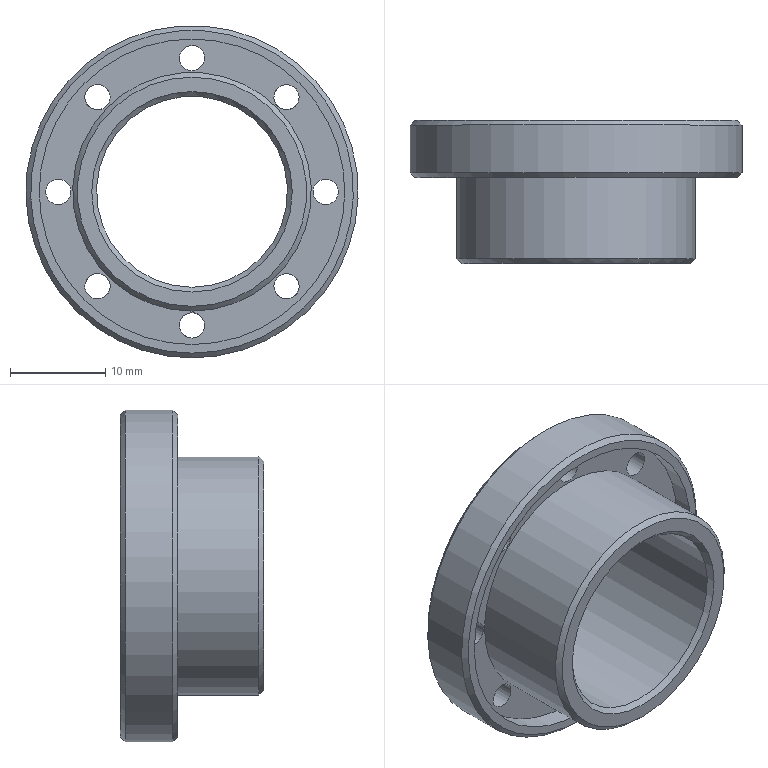Part | NX | features DATUM_CSYS 3, SKETCH 2, EXTRUDE 1, SWP104 1 | 1 solid | 21 faces | box 34.8 x 15 x 34.8 mm | volume 4556 mm3 | cylinder 12 | cone 5 | plane 4 | commonest cylinder face diameters 2.65 x8 20 x1 25 x1 32 x1 34.8 x1
STEP:
#1=CARTESIAN_POINT('',(0.,0.,-10.5));
#2=VERTEX_POINT('',#1);
#3=CARTESIAN_POINT('',(0.,0.,0.));
#4=DIRECTION('',(0.,-1.,0.));
#5=DIRECTION('',(0.,0.,-1.));
#6=AXIS2_PLACEMENT_3D('',#3,#4,#5);
#7=CIRCLE('',#6,10.5);
#8=EDGE_CURVE('',#2,#2,#7,.T.);
#9=ORIENTED_EDGE('',*,*,#8,.F.);
#10=EDGE_LOOP('',(#9));
#11=FACE_BOUND('',#10,.T.);
#12=CARTESIAN_POINT('',(0.,0.,-12.));
#13=VERTEX_POINT('',#12);
#14=CARTESIAN_POINT('',(0.,0.,0.));
#15=DIRECTION('',(0.,-1.,0.));
#16=DIRECTION('',(0.,0.,-1.));
#17=AXIS2_PLACEMENT_3D('',#14,#15,#16);
#18=CIRCLE('',#17,12.);
#19=EDGE_CURVE('',#13,#13,#18,.T.);
#20=ORIENTED_EDGE('',*,*,#19,.T.);
#21=EDGE_LOOP('',(#20));
#22=FACE_BOUND('',#21,.T.);
#23=CARTESIAN_POINT('',(0.,0.,12.));
#24=DIRECTION('',(0.,1.,0.));
#25=DIRECTION('',(0.,0.,1.));
#26=AXIS2_PLACEMENT_3D('',#23,#24,#25);
#27=PLANE('',#26);
#28=ADVANCED_FACE('',(#11,#22),#27,.F.);
#29=CARTESIAN_POINT('',(0.,0.5,-10.));
#30=VERTEX_POINT('',#29);
#31=CARTESIAN_POINT('',(0.,0.5,0.));
#32=DIRECTION('',(0.,-1.,0.));
#33=DIRECTION('',(0.,0.,-1.));
#34=AXIS2_PLACEMENT_3D('',#31,#32,#33);
#35=CIRCLE('',#34,10.);
#36=EDGE_CURVE('',#30,#30,#35,.T.);
#37=ORIENTED_EDGE('',*,*,#36,.F.);
#38=EDGE_LOOP('',(#37));
#39=FACE_BOUND('',#38,.T.);
#40=ORIENTED_EDGE('',*,*,#8,.T.);
#41=EDGE_LOOP('',(#40));
#42=FACE_BOUND('',#41,.T.);
#43=CARTESIAN_POINT('',(0.,0.,0.));
#44=DIRECTION('',(0.,-1.,0.));
#45=DIRECTION('',(0.,0.,-1.));
#46=AXIS2_PLACEMENT_3D('',#43,#44,#45);
#47=CONICAL_SURFACE('',#46,10.5,0.7854);
#48=ADVANCED_FACE('',(#39,#42),#47,.F.);
#49=CARTESIAN_POINT('',(0.,14.5,-10.));
#50=VERTEX_POINT('',#49);
#51=CARTESIAN_POINT('',(0.,14.5,0.));
#52=DIRECTION('',(0.,-1.,0.));
#53=DIRECTION('',(0.,0.,-1.));
#54=AXIS2_PLACEMENT_3D('',#51,#52,#53);
#55=CIRCLE('',#54,10.);
#56=EDGE_CURVE('',#50,#50,#55,.T.);
#57=ORIENTED_EDGE('',*,*,#56,.F.);
#58=EDGE_LOOP('',(#57));
#59=FACE_BOUND('',#58,.T.);
#60=ORIENTED_EDGE('',*,*,#36,.T.);
#61=EDGE_LOOP('',(#60));
#62=FACE_BOUND('',#61,.T.);
#63=CARTESIAN_POINT('',(0.,0.,0.));
#64=DIRECTION('',(0.,-1.,0.));
#65=DIRECTION('',(0.,0.,-1.));
#66=AXIS2_PLACEMENT_3D('',#63,#64,#65);
#67=CYLINDRICAL_SURFACE('',#66,10.);
#68=ADVANCED_FACE('',(#59,#62),#67,.F.);
#69=CARTESIAN_POINT('',(0.,15.,-10.5));
#70=VERTEX_POINT('',#69);
#71=CARTESIAN_POINT('',(0.,15.,0.));
#72=DIRECTION('',(0.,-1.,0.));
#73=DIRECTION('',(0.,0.,-1.));
#74=AXIS2_PLACEMENT_3D('',#71,#72,#73);
#75=CIRCLE('',#74,10.5);
#76=EDGE_CURVE('',#70,#70,#75,.T.);
#77=ORIENTED_EDGE('',*,*,#76,.F.);
#78=EDGE_LOOP('',(#77));
#79=FACE_BOUND('',#78,.T.);
#80=ORIENTED_EDGE('',*,*,#56,.T.);
#81=EDGE_LOOP('',(#80));
#82=FACE_BOUND('',#81,.T.);
#83=CARTESIAN_POINT('',(0.,14.5,0.));
#84=DIRECTION('',(0.,1.,0.));
#85=DIRECTION('',(0.,0.,1.));
#86=AXIS2_PLACEMENT_3D('',#83,#84,#85);
#87=CONICAL_SURFACE('',#86,10.,0.7854);
#88=ADVANCED_FACE('',(#79,#82),#87,.F.);
#89=CARTESIAN_POINT('',(14.,15.,-1.325));
#90=VERTEX_POINT('',#89);
#91=CARTESIAN_POINT('',(14.,15.,0.));
#92=DIRECTION('',(0.,-1.,0.));
#93=DIRECTION('',(0.,0.,-1.));
#94=AXIS2_PLACEMENT_3D('',#91,#92,#93);
#95=CIRCLE('',#94,1.325);
#96=EDGE_CURVE('',#90,#90,#95,.T.);
#97=ORIENTED_EDGE('',*,*,#96,.T.);
#98=EDGE_LOOP('',(#97));
#99=FACE_BOUND('',#98,.T.);
#100=CARTESIAN_POINT('',(9.899,15.,-11.224));
#101=VERTEX_POINT('',#100);
#102=CARTESIAN_POINT('',(9.899,15.,-9.899));
#103=DIRECTION('',(0.,-1.,0.));
#104=DIRECTION('',(0.,0.,-1.));
#105=AXIS2_PLACEMENT_3D('',#102,#103,#104);
#106=CIRCLE('',#105,1.325);
#107=EDGE_CURVE('',#101,#101,#106,.T.);
#108=ORIENTED_EDGE('',*,*,#107,.T.);
#109=EDGE_LOOP('',(#108));
#110=FACE_BOUND('',#109,.T.);
#111=CARTESIAN_POINT('',(0.,15.,-15.325));
#112=VERTEX_POINT('',#111);
#113=CARTESIAN_POINT('',(0.,15.,-14.));
#114=DIRECTION('',(0.,-1.,0.));
#115=DIRECTION('',(0.,0.,-1.));
#116=AXIS2_PLACEMENT_3D('',#113,#114,#115);
#117=CIRCLE('',#116,1.325);
#118=EDGE_CURVE('',#112,#112,#117,.T.);
#119=ORIENTED_EDGE('',*,*,#118,.T.);
#120=EDGE_LOOP('',(#119));
#121=FACE_BOUND('',#120,.T.);
#122=CARTESIAN_POINT('',(-9.899,15.,-11.224));
#123=VERTEX_POINT('',#122);
#124=CARTESIAN_POINT('',(-9.899,15.,-9.899));
#125=DIRECTION('',(0.,-1.,0.));
#126=DIRECTION('',(0.,0.,-1.));
#127=AXIS2_PLACEMENT_3D('',#124,#125,#126);
#128=CIRCLE('',#127,1.325);
#129=EDGE_CURVE('',#123,#123,#128,.T.);
#130=ORIENTED_EDGE('',*,*,#129,.T.);
#131=EDGE_LOOP('',(#130));
#132=FACE_BOUND('',#131,.T.);
#133=CARTESIAN_POINT('',(-14.,15.,-1.325));
#134=VERTEX_POINT('',#133);
#135=CARTESIAN_POINT('',(-14.,15.,0.));
#136=DIRECTION('',(0.,-1.,0.));
#137=DIRECTION('',(0.,0.,-1.));
#138=AXIS2_PLACEMENT_3D('',#135,#136,#137);
#139=CIRCLE('',#138,1.325);
#140=EDGE_CURVE('',#134,#134,#139,.T.);
#141=ORIENTED_EDGE('',*,*,#140,.T.);
#142=EDGE_LOOP('',(#141));
#143=FACE_BOUND('',#142,.T.);
#144=CARTESIAN_POINT('',(-9.899,15.,8.574));
#145=VERTEX_POINT('',#144);
#146=CARTESIAN_POINT('',(-9.899,15.,9.899));
#147=DIRECTION('',(0.,-1.,0.));
#148=DIRECTION('',(0.,0.,-1.));
#149=AXIS2_PLACEMENT_3D('',#146,#147,#148);
#150=CIRCLE('',#149,1.325);
#151=EDGE_CURVE('',#145,#145,#150,.T.);
#152=ORIENTED_EDGE('',*,*,#151,.T.);
#153=EDGE_LOOP('',(#152));
#154=FACE_BOUND('',#153,.T.);
#155=CARTESIAN_POINT('',(0.,15.,12.675));
#156=VERTEX_POINT('',#155);
#157=CARTESIAN_POINT('',(0.,15.,14.));
#158=DIRECTION('',(0.,-1.,0.));
#159=DIRECTION('',(0.,0.,-1.));
#160=AXIS2_PLACEMENT_3D('',#157,#158,#159);
#161=CIRCLE('',#160,1.325);
#162=EDGE_CURVE('',#156,#156,#161,.T.);
#163=ORIENTED_EDGE('',*,*,#162,.T.);
#164=EDGE_LOOP('',(#163));
#165=FACE_BOUND('',#164,.T.);
#166=CARTESIAN_POINT('',(9.899,15.,8.574));
#167=VERTEX_POINT('',#166);
#168=CARTESIAN_POINT('',(9.899,15.,9.899));
#169=DIRECTION('',(0.,-1.,0.));
#170=DIRECTION('',(0.,0.,-1.));
#171=AXIS2_PLACEMENT_3D('',#168,#169,#170);
#172=CIRCLE('',#171,1.325);
#173=EDGE_CURVE('',#167,#167,#172,.T.);
#174=ORIENTED_EDGE('',*,*,#173,.T.);
#175=EDGE_LOOP('',(#174));
#176=FACE_BOUND('',#175,.T.);
#177=CARTESIAN_POINT('',(0.,15.,-16.9));
#178=VERTEX_POINT('',#177);
#179=CARTESIAN_POINT('',(0.,15.,0.));
#180=DIRECTION('',(0.,-1.,0.));
#181=DIRECTION('',(0.,0.,-1.));
#182=AXIS2_PLACEMENT_3D('',#179,#180,#181);
#183=CIRCLE('',#182,16.9);
#184=EDGE_CURVE('',#178,#178,#183,.T.);
#185=ORIENTED_EDGE('',*,*,#184,.F.);
#186=EDGE_LOOP('',(#185));
#187=FACE_BOUND('',#186,.T.);
#188=ORIENTED_EDGE('',*,*,#76,.T.);
#189=EDGE_LOOP('',(#188));
#190=FACE_BOUND('',#189,.T.);
#191=CARTESIAN_POINT('',(0.,15.,10.5));
#192=DIRECTION('',(0.,-1.,0.));
#193=DIRECTION('',(0.,0.,-1.));
#194=AXIS2_PLACEMENT_3D('',#191,#192,#193);
#195=PLANE('',#194);
#196=ADVANCED_FACE('',(#99,#110,#121,#132,#143,#154,#165,#176,#187,#190),#195,.F.);
#197=CARTESIAN_POINT('',(0.,14.5,-17.4));
#198=VERTEX_POINT('',#197);
#199=CARTESIAN_POINT('',(0.,14.5,0.));
#200=DIRECTION('',(0.,-1.,0.));
#201=DIRECTION('',(0.,0.,-1.));
#202=AXIS2_PLACEMENT_3D('',#199,#200,#201);
#203=CIRCLE('',#202,17.4);
#204=EDGE_CURVE('',#198,#198,#203,.T.);
#205=ORIENTED_EDGE('',*,*,#204,.F.);
#206=EDGE_LOOP('',(#205));
#207=FACE_BOUND('',#206,.T.);
#208=ORIENTED_EDGE('',*,*,#184,.T.);
#209=EDGE_LOOP('',(#208));
#210=FACE_BOUND('',#209,.T.);
#211=CARTESIAN_POINT('',(0.,15.,0.));
#212=DIRECTION('',(0.,-1.,0.));
#213=DIRECTION('',(0.,0.,-1.));
#214=AXIS2_PLACEMENT_3D('',#211,#212,#213);
#215=CONICAL_SURFACE('',#214,16.9,0.7854);
#216=ADVANCED_FACE('',(#207,#210),#215,.T.);
#217=CARTESIAN_POINT('',(0.,9.5,-17.4));
#218=VERTEX_POINT('',#217);
#219=CARTESIAN_POINT('',(0.,9.5,0.));
#220=DIRECTION('',(0.,-1.,0.));
#221=DIRECTION('',(0.,0.,-1.));
#222=AXIS2_PLACEMENT_3D('',#219,#220,#221);
#223=CIRCLE('',#222,17.4);
#224=EDGE_CURVE('',#218,#218,#223,.T.);
#225=ORIENTED_EDGE('',*,*,#224,.F.);
#226=EDGE_LOOP('',(#225));
#227=FACE_BOUND('',#226,.T.);
#228=ORIENTED_EDGE('',*,*,#204,.T.);
#229=EDGE_LOOP('',(#228));
#230=FACE_BOUND('',#229,.T.);
#231=CARTESIAN_POINT('',(0.,0.,0.));
#232=DIRECTION('',(0.,-1.,0.));
#233=DIRECTION('',(0.,0.,-1.));
#234=AXIS2_PLACEMENT_3D('',#231,#232,#233);
#235=CYLINDRICAL_SURFACE('',#234,17.4);
#236=ADVANCED_FACE('',(#227,#230),#235,.T.);
#237=CARTESIAN_POINT('',(0.,9.,-16.9));
#238=VERTEX_POINT('',#237);
#239=CARTESIAN_POINT('',(0.,9.,0.));
#240=DIRECTION('',(0.,-1.,0.));
#241=DIRECTION('',(0.,0.,-1.));
#242=AXIS2_PLACEMENT_3D('',#239,#240,#241);
#243=CIRCLE('',#242,16.9);
#244=EDGE_CURVE('',#238,#238,#243,.T.);
#245=ORIENTED_EDGE('',*,*,#244,.F.);
#246=EDGE_LOOP('',(#245));
#247=FACE_BOUND('',#246,.T.);
#248=ORIENTED_EDGE('',*,*,#224,.T.);
#249=EDGE_LOOP('',(#248));
#250=FACE_BOUND('',#249,.T.);
#251=CARTESIAN_POINT('',(0.,9.5,0.));
#252=DIRECTION('',(0.,1.,0.));
#253=DIRECTION('',(0.,0.,1.));
#254=AXIS2_PLACEMENT_3D('',#251,#252,#253);
#255=CONICAL_SURFACE('',#254,17.4,0.7854);
#256=ADVANCED_FACE('',(#247,#250),#255,.T.);
#257=CARTESIAN_POINT('',(0.,9.,-16.));
#258=VERTEX_POINT('',#257);
#259=CARTESIAN_POINT('',(0.,9.,0.));
#260=DIRECTION('',(0.,-1.,0.));
#261=DIRECTION('',(0.,0.,-1.));
#262=AXIS2_PLACEMENT_3D('',#259,#260,#261);
#263=CIRCLE('',#262,16.);
#264=EDGE_CURVE('',#258,#258,#263,.T.);
#265=ORIENTED_EDGE('',*,*,#264,.F.);
#266=EDGE_LOOP('',(#265));
#267=FACE_BOUND('',#266,.T.);
#268=ORIENTED_EDGE('',*,*,#244,.T.);
#269=EDGE_LOOP('',(#268));
#270=FACE_BOUND('',#269,.T.);
#271=CARTESIAN_POINT('',(0.,9.,16.9));
#272=DIRECTION('',(0.,1.,0.));
#273=DIRECTION('',(0.,0.,1.));
#274=AXIS2_PLACEMENT_3D('',#271,#272,#273);
#275=PLANE('',#274);
#276=ADVANCED_FACE('',(#267,#270),#275,.F.);
#277=CARTESIAN_POINT('',(0.,11.,-16.));
#278=VERTEX_POINT('',#277);
#279=CARTESIAN_POINT('',(0.,11.,0.));
#280=DIRECTION('',(0.,-1.,0.));
#281=DIRECTION('',(0.,0.,-1.));
#282=AXIS2_PLACEMENT_3D('',#279,#280,#281);
#283=CIRCLE('',#282,16.);
#284=EDGE_CURVE('',#278,#278,#283,.T.);
#285=ORIENTED_EDGE('',*,*,#284,.F.);
#286=EDGE_LOOP('',(#285));
#287=FACE_BOUND('',#286,.T.);
#288=ORIENTED_EDGE('',*,*,#264,.T.);
#289=EDGE_LOOP('',(#288));
#290=FACE_BOUND('',#289,.T.);
#291=CARTESIAN_POINT('',(0.,0.,0.));
#292=DIRECTION('',(0.,-1.,0.));
#293=DIRECTION('',(0.,0.,-1.));
#294=AXIS2_PLACEMENT_3D('',#291,#292,#293);
#295=CYLINDRICAL_SURFACE('',#294,16.);
#296=ADVANCED_FACE('',(#287,#290),#295,.F.);
#297=CARTESIAN_POINT('',(14.,11.,-1.325));
#298=VERTEX_POINT('',#297);
#299=CARTESIAN_POINT('',(14.,11.,0.));
#300=DIRECTION('',(0.,-1.,0.));
#301=DIRECTION('',(0.,0.,-1.));
#302=AXIS2_PLACEMENT_3D('',#299,#300,#301);
#303=CIRCLE('',#302,1.325);
#304=EDGE_CURVE('',#298,#298,#303,.T.);
#305=ORIENTED_EDGE('',*,*,#304,.F.);
#306=EDGE_LOOP('',(#305));
#307=FACE_BOUND('',#306,.T.);
#308=CARTESIAN_POINT('',(8.963,11.,-10.836));
#309=VERTEX_POINT('',#308);
#310=CARTESIAN_POINT('',(9.899,11.,-9.899));
#311=DIRECTION('',(0.,-1.,0.));
#312=DIRECTION('',(-0.7071,0.,-0.7071));
#313=AXIS2_PLACEMENT_3D('',#310,#311,#312);
#314=CIRCLE('',#313,1.325);
#315=EDGE_CURVE('',#309,#309,#314,.T.);
#316=ORIENTED_EDGE('',*,*,#315,.F.);
#317=EDGE_LOOP('',(#316));
#318=FACE_BOUND('',#317,.T.);
#319=CARTESIAN_POINT('',(-1.325,11.,-14.));
#320=VERTEX_POINT('',#319);
#321=CARTESIAN_POINT('',(0.,11.,-14.));
#322=DIRECTION('',(0.,-1.,0.));
#323=DIRECTION('',(-1.,0.,0.));
#324=AXIS2_PLACEMENT_3D('',#321,#322,#323);
#325=CIRCLE('',#324,1.325);
#326=EDGE_CURVE('',#320,#320,#325,.T.);
#327=ORIENTED_EDGE('',*,*,#326,.F.);
#328=EDGE_LOOP('',(#327));
#329=FACE_BOUND('',#328,.T.);
#330=CARTESIAN_POINT('',(-10.836,11.,-8.963));
#331=VERTEX_POINT('',#330);
#332=CARTESIAN_POINT('',(-9.899,11.,-9.899));
#333=DIRECTION('',(0.,-1.,0.));
#334=DIRECTION('',(-0.7071,0.,0.7071));
#335=AXIS2_PLACEMENT_3D('',#332,#333,#334);
#336=CIRCLE('',#335,1.325);
#337=EDGE_CURVE('',#331,#331,#336,.T.);
#338=ORIENTED_EDGE('',*,*,#337,.F.);
#339=EDGE_LOOP('',(#338));
#340=FACE_BOUND('',#339,.T.);
#341=CARTESIAN_POINT('',(-14.,11.,1.325));
#342=VERTEX_POINT('',#341);
#343=CARTESIAN_POINT('',(-14.,11.,0.));
#344=DIRECTION('',(0.,-1.,0.));
#345=DIRECTION('',(0.,0.,1.));
#346=AXIS2_PLACEMENT_3D('',#343,#344,#345);
#347=CIRCLE('',#346,1.325);
#348=EDGE_CURVE('',#342,#342,#347,.T.);
#349=ORIENTED_EDGE('',*,*,#348,.F.);
#350=EDGE_LOOP('',(#349));
#351=FACE_BOUND('',#350,.T.);
#352=CARTESIAN_POINT('',(-8.963,11.,10.836));
#353=VERTEX_POINT('',#352);
#354=CARTESIAN_POINT('',(-9.899,11.,9.899));
#355=DIRECTION('',(0.,-1.,0.));
#356=DIRECTION('',(0.7071,0.,0.7071));
#357=AXIS2_PLACEMENT_3D('',#354,#355,#356);
#358=CIRCLE('',#357,1.325);
#359=EDGE_CURVE('',#353,#353,#358,.T.);
#360=ORIENTED_EDGE('',*,*,#359,.F.);
#361=EDGE_LOOP('',(#360));
#362=FACE_BOUND('',#361,.T.);
#363=CARTESIAN_POINT('',(1.325,11.,14.));
#364=VERTEX_POINT('',#363);
#365=CARTESIAN_POINT('',(0.,11.,14.));
#366=DIRECTION('',(0.,-1.,0.));
#367=DIRECTION('',(1.,0.,0.));
#368=AXIS2_PLACEMENT_3D('',#365,#366,#367);
#369=CIRCLE('',#368,1.325);
#370=EDGE_CURVE('',#364,#364,#369,.T.);
#371=ORIENTED_EDGE('',*,*,#370,.F.);
#372=EDGE_LOOP('',(#371));
#373=FACE_BOUND('',#372,.T.);
#374=CARTESIAN_POINT('',(10.836,11.,8.963));
#375=VERTEX_POINT('',#374);
#376=CARTESIAN_POINT('',(9.899,11.,9.899));
#377=DIRECTION('',(0.,-1.,0.));
#378=DIRECTION('',(0.7071,0.,-0.7071));
#379=AXIS2_PLACEMENT_3D('',#376,#377,#378);
#380=CIRCLE('',#379,1.325);
#381=EDGE_CURVE('',#375,#375,#380,.T.);
#382=ORIENTED_EDGE('',*,*,#381,.F.);
#383=EDGE_LOOP('',(#382));
#384=FACE_BOUND('',#383,.T.);
#385=CARTESIAN_POINT('',(0.,11.,-12.5));
#386=VERTEX_POINT('',#385);
#387=CARTESIAN_POINT('',(0.,11.,0.));
#388=DIRECTION('',(0.,-1.,0.));
#389=DIRECTION('',(0.,0.,-1.));
#390=AXIS2_PLACEMENT_3D('',#387,#388,#389);
#391=CIRCLE('',#390,12.5);
#392=EDGE_CURVE('',#386,#386,#391,.T.);
#393=ORIENTED_EDGE('',*,*,#392,.F.);
#394=EDGE_LOOP('',(#393));
#395=FACE_BOUND('',#394,.T.);
#396=ORIENTED_EDGE('',*,*,#284,.T.);
#397=EDGE_LOOP('',(#396));
#398=FACE_BOUND('',#397,.T.);
#399=CARTESIAN_POINT('',(0.,11.,16.));
#400=DIRECTION('',(0.,1.,0.));
#401=DIRECTION('',(0.,0.,1.));
#402=AXIS2_PLACEMENT_3D('',#399,#400,#401);
#403=PLANE('',#402);
#404=ADVANCED_FACE('',(#307,#318,#329,#340,#351,#362,#373,#384,#395,#398),#403,.F.);
#405=CARTESIAN_POINT('',(0.,0.5,-12.5));
#406=VERTEX_POINT('',#405);
#407=CARTESIAN_POINT('',(0.,0.5,0.));
#408=DIRECTION('',(0.,-1.,0.));
#409=DIRECTION('',(0.,0.,-1.));
#410=AXIS2_PLACEMENT_3D('',#407,#408,#409);
#411=CIRCLE('',#410,12.5);
#412=EDGE_CURVE('',#406,#406,#411,.T.);
#413=ORIENTED_EDGE('',*,*,#412,.F.);
#414=EDGE_LOOP('',(#413));
#415=FACE_BOUND('',#414,.T.);
#416=ORIENTED_EDGE('',*,*,#392,.T.);
#417=EDGE_LOOP('',(#416));
#418=FACE_BOUND('',#417,.T.);
#419=CARTESIAN_POINT('',(0.,0.,0.));
#420=DIRECTION('',(0.,-1.,0.));
#421=DIRECTION('',(0.,0.,-1.));
#422=AXIS2_PLACEMENT_3D('',#419,#420,#421);
#423=CYLINDRICAL_SURFACE('',#422,12.5);
#424=ADVANCED_FACE('',(#415,#418),#423,.T.);
#425=ORIENTED_EDGE('',*,*,#19,.F.);
#426=EDGE_LOOP('',(#425));
#427=FACE_BOUND('',#426,.T.);
#428=ORIENTED_EDGE('',*,*,#412,.T.);
#429=EDGE_LOOP('',(#428));
#430=FACE_BOUND('',#429,.T.);
#431=CARTESIAN_POINT('',(0.,0.5,0.));
#432=DIRECTION('',(0.,1.,0.));
#433=DIRECTION('',(0.,0.,1.));
#434=AXIS2_PLACEMENT_3D('',#431,#432,#433);
#435=CONICAL_SURFACE('',#434,12.5,0.7854);
#436=ADVANCED_FACE('',(#427,#430),#435,.T.);
#437=ORIENTED_EDGE('',*,*,#381,.T.);
#438=EDGE_LOOP('',(#437));
#439=FACE_BOUND('',#438,.T.);
#440=ORIENTED_EDGE('',*,*,#173,.F.);
#441=EDGE_LOOP('',(#440));
#442=FACE_BOUND('',#441,.T.);
#443=CARTESIAN_POINT('',(9.899,30.,9.899));
#444=DIRECTION('',(0.,-1.,0.));
#445=DIRECTION('',(0.,0.,-1.));
#446=AXIS2_PLACEMENT_3D('',#443,#444,#445);
#447=CYLINDRICAL_SURFACE('',#446,1.325);
#448=ADVANCED_FACE('',(#439,#442),#447,.F.);
#449=ORIENTED_EDGE('',*,*,#370,.T.);
#450=EDGE_LOOP('',(#449));
#451=FACE_BOUND('',#450,.T.);
#452=ORIENTED_EDGE('',*,*,#162,.F.);
#453=EDGE_LOOP('',(#452));
#454=FACE_BOUND('',#453,.T.);
#455=CARTESIAN_POINT('',(0.,30.,14.));
#456=DIRECTION('',(0.,-1.,0.));
#457=DIRECTION('',(0.,0.,-1.));
#458=AXIS2_PLACEMENT_3D('',#455,#456,#457);
#459=CYLINDRICAL_SURFACE('',#458,1.325);
#460=ADVANCED_FACE('',(#451,#454),#459,.F.);
#461=ORIENTED_EDGE('',*,*,#359,.T.);
#462=EDGE_LOOP('',(#461));
#463=FACE_BOUND('',#462,.T.);
#464=ORIENTED_EDGE('',*,*,#151,.F.);
#465=EDGE_LOOP('',(#464));
#466=FACE_BOUND('',#465,.T.);
#467=CARTESIAN_POINT('',(-9.899,30.,9.899));
#468=DIRECTION('',(0.,-1.,0.));
#469=DIRECTION('',(0.,0.,-1.));
#470=AXIS2_PLACEMENT_3D('',#467,#468,#469);
#471=CYLINDRICAL_SURFACE('',#470,1.325);
#472=ADVANCED_FACE('',(#463,#466),#471,.F.);
#473=ORIENTED_EDGE('',*,*,#348,.T.);
#474=EDGE_LOOP('',(#473));
#475=FACE_BOUND('',#474,.T.);
#476=ORIENTED_EDGE('',*,*,#140,.F.);
#477=EDGE_LOOP('',(#476));
#478=FACE_BOUND('',#477,.T.);
#479=CARTESIAN_POINT('',(-14.,30.,0.));
#480=DIRECTION('',(0.,-1.,0.));
#481=DIRECTION('',(0.,0.,-1.));
#482=AXIS2_PLACEMENT_3D('',#479,#480,#481);
#483=CYLINDRICAL_SURFACE('',#482,1.325);
#484=ADVANCED_FACE('',(#475,#478),#483,.F.);
#485=ORIENTED_EDGE('',*,*,#337,.T.);
#486=EDGE_LOOP('',(#485));
#487=FACE_BOUND('',#486,.T.);
#488=ORIENTED_EDGE('',*,*,#129,.F.);
#489=EDGE_LOOP('',(#488));
#490=FACE_BOUND('',#489,.T.);
#491=CARTESIAN_POINT('',(-9.899,30.,-9.899));
#492=DIRECTION('',(0.,-1.,0.));
#493=DIRECTION('',(0.,0.,-1.));
#494=AXIS2_PLACEMENT_3D('',#491,#492,#493);
#495=CYLINDRICAL_SURFACE('',#494,1.325);
#496=ADVANCED_FACE('',(#487,#490),#495,.F.);
#497=ORIENTED_EDGE('',*,*,#326,.T.);
#498=EDGE_LOOP('',(#497));
#499=FACE_BOUND('',#498,.T.);
#500=ORIENTED_EDGE('',*,*,#118,.F.);
#501=EDGE_LOOP('',(#500));
#502=FACE_BOUND('',#501,.T.);
#503=CARTESIAN_POINT('',(0.,30.,-14.));
#504=DIRECTION('',(0.,-1.,0.));
#505=DIRECTION('',(0.,0.,-1.));
#506=AXIS2_PLACEMENT_3D('',#503,#504,#505);
#507=CYLINDRICAL_SURFACE('',#506,1.325);
#508=ADVANCED_FACE('',(#499,#502),#507,.F.);
#509=ORIENTED_EDGE('',*,*,#315,.T.);
#510=EDGE_LOOP('',(#509));
#511=FACE_BOUND('',#510,.T.);
#512=ORIENTED_EDGE('',*,*,#107,.F.);
#513=EDGE_LOOP('',(#512));
#514=FACE_BOUND('',#513,.T.);
#515=CARTESIAN_POINT('',(9.899,30.,-9.899));
#516=DIRECTION('',(0.,-1.,0.));
#517=DIRECTION('',(0.,0.,-1.));
#518=AXIS2_PLACEMENT_3D('',#515,#516,#517);
#519=CYLINDRICAL_SURFACE('',#518,1.325);
#520=ADVANCED_FACE('',(#511,#514),#519,.F.);
#521=ORIENTED_EDGE('',*,*,#304,.T.);
#522=EDGE_LOOP('',(#521));
#523=FACE_BOUND('',#522,.T.);
#524=ORIENTED_EDGE('',*,*,#96,.F.);
#525=EDGE_LOOP('',(#524));
#526=FACE_BOUND('',#525,.T.);
#527=CARTESIAN_POINT('',(14.,30.,0.));
#528=DIRECTION('',(0.,-1.,0.));
#529=DIRECTION('',(0.,0.,-1.));
#530=AXIS2_PLACEMENT_3D('',#527,#528,#529);
#531=CYLINDRICAL_SURFACE('',#530,1.325);
#532=ADVANCED_FACE('',(#523,#526),#531,.F.);
#533=CLOSED_SHELL('',(#28,#48,#68,#88,#196,#216,#236,#256,#276,#296,#404,#424,#436,#448,#460,#472,#484,#496,#508,#520,#532));
#534=MANIFOLD_SOLID_BREP('',#533);
#535=(LENGTH_UNIT()NAMED_UNIT(*)SI_UNIT(.MILLI.,.METRE.));
#536=UNCERTAINTY_MEASURE_WITH_UNIT(LENGTH_MEASURE(0.00001),#535,'','');
#537=(NAMED_UNIT(*)PLANE_ANGLE_UNIT()SI_UNIT($,.RADIAN.));
#538=(NAMED_UNIT(*)SI_UNIT($,.STERADIAN.)SOLID_ANGLE_UNIT());
#539=(GEOMETRIC_REPRESENTATION_CONTEXT(3)GLOBAL_UNCERTAINTY_ASSIGNED_CONTEXT((#536))GLOBAL_UNIT_ASSIGNED_CONTEXT((#535,#537,#538))REPRESENTATION_CONTEXT('',''));
#540=ADVANCED_BREP_SHAPE_REPRESENTATION('',(#534),#539);